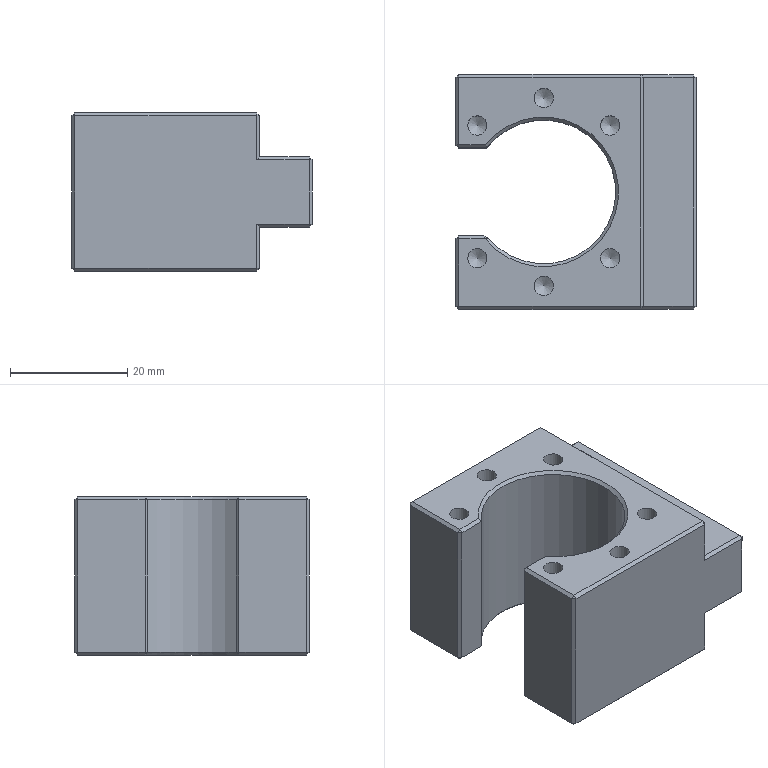Part | 1 solid | 77 faces | box 41 x 40 x 27 mm | volume 24086 mm3 | plane 62 | cone 8 | cylinder 7 | commonest cylinder face diameters 3.3 x6 24.5 x1